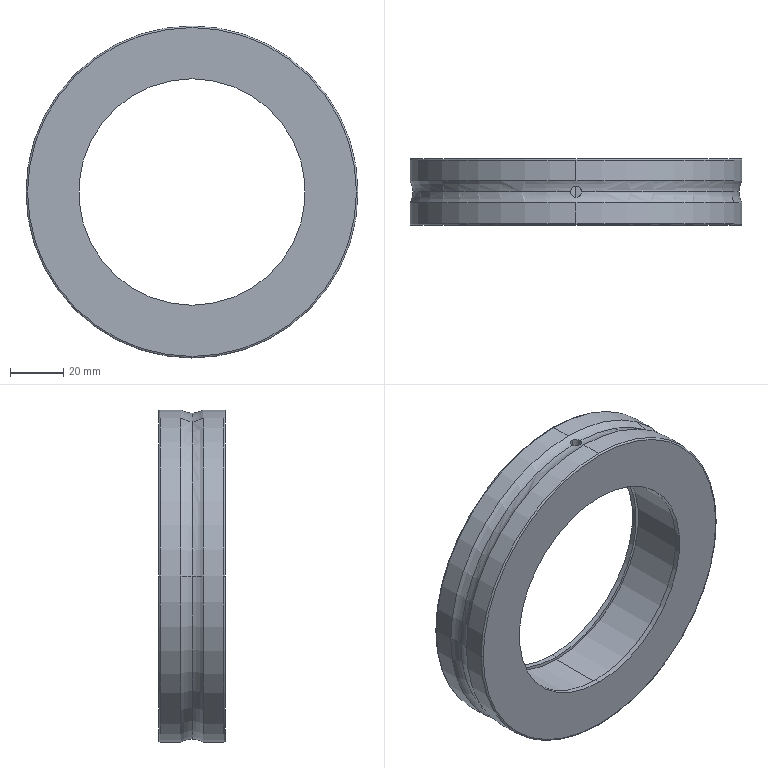Part | SolidWorks | features BaseBody 1 | 1 solid | 24 faces | box 125 x 25 x 125 mm | volume 154919 mm3 | cylinder 12 | torus 8 | plane 4 | commonest cylinder face diameters 85.25 x4 125 x4 4.159 x2 87.5 x2
STEP:
#1=CARTESIAN_POINT('',(-2132.95,755.069,-1534.999));
#2=VERTEX_POINT('',#1);
#3=CARTESIAN_POINT('',(-2132.95,755.069,-1620.249));
#4=VERTEX_POINT('',#3);
#5=CARTESIAN_POINT('',(-2132.95,755.069,-1577.624));
#6=DIRECTION('',(0.,-1.,0.));
#7=DIRECTION('',(0.,0.,1.));
#8=AXIS2_PLACEMENT_3D('',#5,#6,#7);
#9=CIRCLE('',#8,42.625);
#10=EDGE_CURVE('',#2,#4,#9,.T.);
#11=ORIENTED_EDGE('',*,*,#10,.F.);
#12=CARTESIAN_POINT('',(-2132.95,755.069,-1577.624));
#13=DIRECTION('',(0.,-1.,0.));
#14=DIRECTION('',(0.,0.,-1.));
#15=AXIS2_PLACEMENT_3D('',#12,#13,#14);
#16=CIRCLE('',#15,42.625);
#17=EDGE_CURVE('',#4,#2,#16,.T.);
#18=ORIENTED_EDGE('',*,*,#17,.F.);
#19=EDGE_LOOP('',(#11,#18));
#20=FACE_BOUND('',#19,.T.);
#21=CARTESIAN_POINT('',(-2071.05,755.069,-1577.624));
#22=VERTEX_POINT('',#21);
#23=CARTESIAN_POINT('',(-2194.85,755.069,-1577.624));
#24=VERTEX_POINT('',#23);
#25=CARTESIAN_POINT('',(-2132.95,755.069,-1577.624));
#26=DIRECTION('',(0.,-1.,0.));
#27=DIRECTION('',(0.,0.,1.));
#28=AXIS2_PLACEMENT_3D('',#25,#26,#27);
#29=CIRCLE('',#28,61.9);
#30=EDGE_CURVE('',#22,#24,#29,.T.);
#31=ORIENTED_EDGE('',*,*,#30,.T.);
#32=CARTESIAN_POINT('',(-2132.95,755.069,-1577.624));
#33=DIRECTION('',(0.,-1.,0.));
#34=DIRECTION('',(-1.,0.,0.));
#35=AXIS2_PLACEMENT_3D('',#32,#33,#34);
#36=CIRCLE('',#35,61.9);
#37=EDGE_CURVE('',#24,#22,#36,.T.);
#38=ORIENTED_EDGE('',*,*,#37,.T.);
#39=EDGE_LOOP('',(#31,#38));
#40=FACE_OUTER_BOUND('',#39,.T.);
#41=CARTESIAN_POINT('',(-2064.86,755.069,-1645.714));
#42=DIRECTION('',(0.,-1.,0.));
#43=DIRECTION('',(0.,0.,-1.));
#44=AXIS2_PLACEMENT_3D('',#41,#42,#43);
#45=PLANE('',#44);
#46=ADVANCED_FACE('',(#20,#40),#45,.T.);
#47=CARTESIAN_POINT('',(-2070.45,755.669,-1577.624));
#48=VERTEX_POINT('',#47);
#49=CARTESIAN_POINT('',(-2071.05,755.669,-1577.624));
#50=DIRECTION('',(0.,0.,-1.));
#51=DIRECTION('',(1.,0.,0.));
#52=AXIS2_PLACEMENT_3D('',#49,#50,#51);
#53=CIRCLE('',#52,0.6);
#54=EDGE_CURVE('',#48,#22,#53,.T.);
#55=ORIENTED_EDGE('',*,*,#54,.T.);
#56=ORIENTED_EDGE('',*,*,#37,.F.);
#57=CARTESIAN_POINT('',(-2195.45,755.669,-1577.624));
#58=VERTEX_POINT('',#57);
#59=CARTESIAN_POINT('',(-2194.85,755.669,-1577.624));
#60=DIRECTION('',(0.,0.,-1.));
#61=DIRECTION('',(0.,-1.,0.));
#62=AXIS2_PLACEMENT_3D('',#59,#60,#61);
#63=CIRCLE('',#62,0.6);
#64=EDGE_CURVE('',#24,#58,#63,.T.);
#65=ORIENTED_EDGE('',*,*,#64,.T.);
#66=CARTESIAN_POINT('',(-2132.95,755.669,-1640.124));
#67=VERTEX_POINT('',#66);
#68=CARTESIAN_POINT('',(-2132.95,755.669,-1577.624));
#69=DIRECTION('',(0.,-1.,0.));
#70=DIRECTION('',(-1.,0.,0.));
#71=AXIS2_PLACEMENT_3D('',#68,#69,#70);
#72=CIRCLE('',#71,62.5);
#73=EDGE_CURVE('',#58,#67,#72,.T.);
#74=ORIENTED_EDGE('',*,*,#73,.T.);
#75=CARTESIAN_POINT('',(-2132.95,755.669,-1577.624));
#76=DIRECTION('',(0.,-1.,0.));
#77=DIRECTION('',(0.,0.,-1.));
#78=AXIS2_PLACEMENT_3D('',#75,#76,#77);
#79=CIRCLE('',#78,62.5);
#80=EDGE_CURVE('',#67,#48,#79,.T.);
#81=ORIENTED_EDGE('',*,*,#80,.T.);
#82=EDGE_LOOP('',(#55,#56,#65,#74,#81));
#83=FACE_OUTER_BOUND('',#82,.T.);
#84=CARTESIAN_POINT('',(-2132.95,755.669,-1577.624));
#85=DIRECTION('',(0.,-1.,0.));
#86=DIRECTION('',(-0.9962,0.,0.08716));
#87=AXIS2_PLACEMENT_3D('',#84,#85,#86);
#88=TOROIDAL_SURFACE('',#87,61.9,0.6);
#89=ADVANCED_FACE('',(#83),#88,.T.);
#90=CARTESIAN_POINT('',(-2132.95,763.41,-1515.124));
#91=VERTEX_POINT('',#90);
#92=CARTESIAN_POINT('',(-2132.95,755.669,-1515.124));
#93=VERTEX_POINT('',#92);
#94=CARTESIAN_POINT('',(-2132.95,763.41,-1515.124));
#95=DIRECTION('',(0.,-1.,0.));
#96=VECTOR('',#95,1000.);
#97=LINE('',#94,#96);
#98=EDGE_CURVE('',#91,#93,#97,.T.);
#99=ORIENTED_EDGE('',*,*,#98,.T.);
#100=CARTESIAN_POINT('',(-2132.95,755.669,-1577.624));
#101=DIRECTION('',(0.,-1.,0.));
#102=DIRECTION('',(1.,0.,0.));
#103=AXIS2_PLACEMENT_3D('',#100,#101,#102);
#104=CIRCLE('',#103,62.5);
#105=EDGE_CURVE('',#48,#93,#104,.T.);
#106=ORIENTED_EDGE('',*,*,#105,.F.);
#107=ORIENTED_EDGE('',*,*,#80,.F.);
#108=CARTESIAN_POINT('',(-2132.95,763.41,-1640.124));
#109=VERTEX_POINT('',#108);
#110=CARTESIAN_POINT('',(-2132.95,755.669,-1640.124));
#111=DIRECTION('',(0.,1.,0.));
#112=VECTOR('',#111,1000.);
#113=LINE('',#110,#112);
#114=EDGE_CURVE('',#67,#109,#113,.T.);
#115=ORIENTED_EDGE('',*,*,#114,.T.);
#116=CARTESIAN_POINT('',(-2070.45,763.41,-1577.624));
#117=VERTEX_POINT('',#116);
#118=CARTESIAN_POINT('',(-2132.95,763.41,-1577.624));
#119=DIRECTION('',(0.,-1.,0.));
#120=DIRECTION('',(0.,0.,-1.));
#121=AXIS2_PLACEMENT_3D('',#118,#119,#120);
#122=CIRCLE('',#121,62.5);
#123=EDGE_CURVE('',#109,#117,#122,.T.);
#124=ORIENTED_EDGE('',*,*,#123,.T.);
#125=CARTESIAN_POINT('',(-2132.95,763.41,-1577.624));
#126=DIRECTION('',(0.,-1.,0.));
#127=DIRECTION('',(1.,0.,0.));
#128=AXIS2_PLACEMENT_3D('',#125,#126,#127);
#129=CIRCLE('',#128,62.5);
#130=EDGE_CURVE('',#117,#91,#129,.T.);
#131=ORIENTED_EDGE('',*,*,#130,.T.);
#132=EDGE_LOOP('',(#99,#106,#107,#115,#124,#131));
#133=FACE_OUTER_BOUND('',#132,.T.);
#134=CARTESIAN_POINT('',(-2132.95,763.797,-1577.624));
#135=DIRECTION('',(0.,1.,0.));
#136=DIRECTION('',(-0.08716,0.,0.9962));
#137=AXIS2_PLACEMENT_3D('',#134,#135,#136);
#138=CYLINDRICAL_SURFACE('',#137,62.5);
#139=ADVANCED_FACE('',(#133),#138,.T.);
#140=CARTESIAN_POINT('',(-2194.325,767.569,-1577.624));
#141=VERTEX_POINT('',#140);
#142=CARTESIAN_POINT('',(-2135.029,767.569,-1516.285));
#143=VERTEX_POINT('',#142);
#144=CARTESIAN_POINT('',(-2132.95,767.569,-1577.624));
#145=DIRECTION('',(0.,1.,0.));
#146=DIRECTION('',(-1.,0.,0.));
#147=AXIS2_PLACEMENT_3D('',#144,#145,#146);
#148=CIRCLE('',#147,61.375);
#149=EDGE_CURVE('',#141,#143,#148,.T.);
#150=ORIENTED_EDGE('',*,*,#149,.T.);
#151=CARTESIAN_POINT('',(-2132.95,769.648,-1515.983));
#152=VERTEX_POINT('',#151);
#153=CARTESIAN_POINT('',(-2135.029,767.569,-1516.285));
#154=CARTESIAN_POINT('',(-2135.029,767.706,-1516.285));
#155=CARTESIAN_POINT('',(-2135.016,767.842,-1516.281));
#156=CARTESIAN_POINT('',(-2134.963,768.108,-1516.266));
#157=CARTESIAN_POINT('',(-2134.923,768.239,-1516.255));
#158=CARTESIAN_POINT('',(-2134.765,768.62,-1516.213));
#159=CARTESIAN_POINT('',(-2134.616,768.843,-1516.175));
#160=CARTESIAN_POINT('',(-2134.323,769.136,-1516.115));
#161=CARTESIAN_POINT('',(-2134.218,769.222,-1516.095));
#162=CARTESIAN_POINT('',(-2133.994,769.372,-1516.059));
#163=CARTESIAN_POINT('',(-2133.876,769.436,-1516.042));
#164=CARTESIAN_POINT('',(-2133.491,769.595,-1515.999));
#165=CARTESIAN_POINT('',(-2133.225,769.648,-1515.983));
#166=CARTESIAN_POINT('',(-2132.95,769.648,-1515.983));
#167=B_SPLINE_CURVE_WITH_KNOTS('',3,(#153,#154,#155,#156,#157,#158,#159,#160,#161,#162,#163,#164,#165,#166),.UNSPECIFIED.,.F.,.F.,(4,2,2,2,2,2,4),(0.,0.125,0.25,0.5,0.625,0.75,1.),.UNSPECIFIED.);
#168=EDGE_CURVE('',#143,#152,#167,.T.);
#169=ORIENTED_EDGE('',*,*,#168,.T.);
#170=CARTESIAN_POINT('',(-2130.87,767.569,-1516.285));
#171=VERTEX_POINT('',#170);
#172=CARTESIAN_POINT('',(-2132.95,769.648,-1515.983));
#173=CARTESIAN_POINT('',(-2132.812,769.648,-1515.983));
#174=CARTESIAN_POINT('',(-2132.677,769.635,-1515.987));
#175=CARTESIAN_POINT('',(-2132.411,769.582,-1516.002));
#176=CARTESIAN_POINT('',(-2132.279,769.542,-1516.014));
#177=CARTESIAN_POINT('',(-2131.899,769.384,-1516.056));
#178=CARTESIAN_POINT('',(-2131.674,769.233,-1516.095));
#179=CARTESIAN_POINT('',(-2131.284,768.844,-1516.175));
#180=CARTESIAN_POINT('',(-2131.135,768.622,-1516.213));
#181=CARTESIAN_POINT('',(-2130.923,768.11,-1516.269));
#182=CARTESIAN_POINT('',(-2130.87,767.844,-1516.285));
#183=CARTESIAN_POINT('',(-2130.87,767.569,-1516.285));
#184=B_SPLINE_CURVE_WITH_KNOTS('',3,(#172,#173,#174,#175,#176,#177,#178,#179,#180,#181,#182,#183),.UNSPECIFIED.,.F.,.F.,(4,2,2,2,2,4),(0.,0.125,0.25,0.5,0.75,1.),.UNSPECIFIED.);
#185=EDGE_CURVE('',#152,#171,#184,.T.);
#186=ORIENTED_EDGE('',*,*,#185,.T.);
#187=CARTESIAN_POINT('',(-2071.575,767.569,-1577.624));
#188=VERTEX_POINT('',#187);
#189=CARTESIAN_POINT('',(-2132.95,767.569,-1577.624));
#190=DIRECTION('',(0.,1.,0.));
#191=DIRECTION('',(0.03388,0.,0.9994));
#192=AXIS2_PLACEMENT_3D('',#189,#190,#191);
#193=CIRCLE('',#192,61.375);
#194=EDGE_CURVE('',#171,#188,#193,.T.);
#195=ORIENTED_EDGE('',*,*,#194,.T.);
#196=CARTESIAN_POINT('',(-2070.45,771.727,-1577.624));
#197=VERTEX_POINT('',#196);
#198=CARTESIAN_POINT('',(-2063.325,767.569,-1577.624));
#199=DIRECTION('',(0.,0.,-1.));
#200=DIRECTION('',(-1.,0.,0.));
#201=AXIS2_PLACEMENT_3D('',#198,#199,#200);
#202=CIRCLE('',#201,8.25);
#203=EDGE_CURVE('',#188,#197,#202,.T.);
#204=ORIENTED_EDGE('',*,*,#203,.T.);
#205=CARTESIAN_POINT('',(-2132.95,771.727,-1515.124));
#206=VERTEX_POINT('',#205);
#207=CARTESIAN_POINT('',(-2132.95,771.727,-1577.624));
#208=DIRECTION('',(0.,-1.,0.));
#209=DIRECTION('',(1.,0.,0.));
#210=AXIS2_PLACEMENT_3D('',#207,#208,#209);
#211=CIRCLE('',#210,62.5);
#212=EDGE_CURVE('',#197,#206,#211,.T.);
#213=ORIENTED_EDGE('',*,*,#212,.T.);
#214=CARTESIAN_POINT('',(-2195.45,771.727,-1577.624));
#215=VERTEX_POINT('',#214);
#216=CARTESIAN_POINT('',(-2132.95,771.727,-1577.624));
#217=DIRECTION('',(0.,-1.,0.));
#218=DIRECTION('',(0.,0.,1.));
#219=AXIS2_PLACEMENT_3D('',#216,#217,#218);
#220=CIRCLE('',#219,62.5);
#221=EDGE_CURVE('',#206,#215,#220,.T.);
#222=ORIENTED_EDGE('',*,*,#221,.T.);
#223=CARTESIAN_POINT('',(-2202.575,767.569,-1577.624));
#224=DIRECTION('',(0.,0.,-1.));
#225=DIRECTION('',(0.8636,0.5041,0.));
#226=AXIS2_PLACEMENT_3D('',#223,#224,#225);
#227=CIRCLE('',#226,8.25);
#228=EDGE_CURVE('',#215,#141,#227,.T.);
#229=ORIENTED_EDGE('',*,*,#228,.T.);
#230=EDGE_LOOP('',(#150,#169,#186,#195,#204,#213,#222,#229));
#231=FACE_OUTER_BOUND('',#230,.T.);
#232=CARTESIAN_POINT('',(-2132.95,767.569,-1577.624));
#233=DIRECTION('',(0.,-1.,0.));
#234=DIRECTION('',(0.9962,0.,-0.08716));
#235=AXIS2_PLACEMENT_3D('',#232,#233,#234);
#236=TOROIDAL_SURFACE('',#235,69.625,8.25);
#237=ADVANCED_FACE('',(#231),#236,.F.);
#238=CARTESIAN_POINT('',(-2132.95,779.469,-1515.124));
#239=VERTEX_POINT('',#238);
#240=CARTESIAN_POINT('',(-2132.95,779.469,-1515.124));
#241=DIRECTION('',(0.,-1.,0.));
#242=VECTOR('',#241,1000.);
#243=LINE('',#240,#242);
#244=EDGE_CURVE('',#239,#206,#243,.T.);
#245=ORIENTED_EDGE('',*,*,#244,.T.);
#246=ORIENTED_EDGE('',*,*,#212,.F.);
#247=CARTESIAN_POINT('',(-2132.95,771.727,-1640.124));
#248=VERTEX_POINT('',#247);
#249=CARTESIAN_POINT('',(-2132.95,771.727,-1577.624));
#250=DIRECTION('',(0.,-1.,0.));
#251=DIRECTION('',(0.,0.,-1.));
#252=AXIS2_PLACEMENT_3D('',#249,#250,#251);
#253=CIRCLE('',#252,62.5);
#254=EDGE_CURVE('',#248,#197,#253,.T.);
#255=ORIENTED_EDGE('',*,*,#254,.F.);
#256=CARTESIAN_POINT('',(-2132.95,779.469,-1640.124));
#257=VERTEX_POINT('',#256);
#258=CARTESIAN_POINT('',(-2132.95,771.727,-1640.124));
#259=DIRECTION('',(0.,1.,0.));
#260=VECTOR('',#259,1000.);
#261=LINE('',#258,#260);
#262=EDGE_CURVE('',#248,#257,#261,.T.);
#263=ORIENTED_EDGE('',*,*,#262,.T.);
#264=CARTESIAN_POINT('',(-2070.45,779.469,-1577.624));
#265=VERTEX_POINT('',#264);
#266=CARTESIAN_POINT('',(-2132.95,779.469,-1577.624));
#267=DIRECTION('',(0.,-1.,0.));
#268=DIRECTION('',(0.,0.,-1.));
#269=AXIS2_PLACEMENT_3D('',#266,#267,#268);
#270=CIRCLE('',#269,62.5);
#271=EDGE_CURVE('',#257,#265,#270,.T.);
#272=ORIENTED_EDGE('',*,*,#271,.T.);
#273=CARTESIAN_POINT('',(-2132.95,779.469,-1577.624));
#274=DIRECTION('',(0.,-1.,0.));
#275=DIRECTION('',(1.,0.,0.));
#276=AXIS2_PLACEMENT_3D('',#273,#274,#275);
#277=CIRCLE('',#276,62.5);
#278=EDGE_CURVE('',#265,#239,#277,.T.);
#279=ORIENTED_EDGE('',*,*,#278,.T.);
#280=EDGE_LOOP('',(#245,#246,#255,#263,#272,#279));
#281=FACE_OUTER_BOUND('',#280,.T.);
#282=CARTESIAN_POINT('',(-2132.95,779.856,-1577.624));
#283=DIRECTION('',(0.,1.,0.));
#284=DIRECTION('',(-0.08716,0.,0.9962));
#285=AXIS2_PLACEMENT_3D('',#282,#283,#284);
#286=CYLINDRICAL_SURFACE('',#285,62.5);
#287=ADVANCED_FACE('',(#281),#286,.T.);
#288=CARTESIAN_POINT('',(-2071.05,780.069,-1577.624));
#289=VERTEX_POINT('',#288);
#290=CARTESIAN_POINT('',(-2071.05,779.469,-1577.624));
#291=DIRECTION('',(0.,0.,-1.));
#292=DIRECTION('',(0.,1.,0.));
#293=AXIS2_PLACEMENT_3D('',#290,#291,#292);
#294=CIRCLE('',#293,0.6);
#295=EDGE_CURVE('',#289,#265,#294,.T.);
#296=ORIENTED_EDGE('',*,*,#295,.T.);
#297=ORIENTED_EDGE('',*,*,#271,.F.);
#298=CARTESIAN_POINT('',(-2195.45,779.469,-1577.624));
#299=VERTEX_POINT('',#298);
#300=CARTESIAN_POINT('',(-2132.95,779.469,-1577.624));
#301=DIRECTION('',(0.,-1.,0.));
#302=DIRECTION('',(-1.,0.,0.));
#303=AXIS2_PLACEMENT_3D('',#300,#301,#302);
#304=CIRCLE('',#303,62.5);
#305=EDGE_CURVE('',#299,#257,#304,.T.);
#306=ORIENTED_EDGE('',*,*,#305,.F.);
#307=CARTESIAN_POINT('',(-2194.85,780.069,-1577.624));
#308=VERTEX_POINT('',#307);
#309=CARTESIAN_POINT('',(-2194.85,779.469,-1577.624));
#310=DIRECTION('',(0.,0.,-1.));
#311=DIRECTION('',(-1.,0.,0.));
#312=AXIS2_PLACEMENT_3D('',#309,#310,#311);
#313=CIRCLE('',#312,0.6);
#314=EDGE_CURVE('',#299,#308,#313,.T.);
#315=ORIENTED_EDGE('',*,*,#314,.T.);
#316=CARTESIAN_POINT('',(-2132.95,780.069,-1577.624));
#317=DIRECTION('',(0.,1.,0.));
#318=DIRECTION('',(1.,0.,0.));
#319=AXIS2_PLACEMENT_3D('',#316,#317,#318);
#320=CIRCLE('',#319,61.9);
#321=EDGE_CURVE('',#289,#308,#320,.T.);
#322=ORIENTED_EDGE('',*,*,#321,.F.);
#323=EDGE_LOOP('',(#296,#297,#306,#315,#322));
#324=FACE_OUTER_BOUND('',#323,.T.);
#325=CARTESIAN_POINT('',(-2132.95,779.469,-1577.624));
#326=DIRECTION('',(0.,-1.,0.));
#327=DIRECTION('',(-0.9962,0.,0.08716));
#328=AXIS2_PLACEMENT_3D('',#325,#326,#327);
#329=TOROIDAL_SURFACE('',#328,61.9,0.6);
#330=ADVANCED_FACE('',(#324),#329,.T.);
#331=CARTESIAN_POINT('',(-2132.95,780.069,-1620.249));
#332=VERTEX_POINT('',#331);
#333=CARTESIAN_POINT('',(-2132.95,780.069,-1534.999));
#334=VERTEX_POINT('',#333);
#335=CARTESIAN_POINT('',(-2132.95,780.069,-1577.624));
#336=DIRECTION('',(0.,1.,0.));
#337=DIRECTION('',(0.,0.,-1.));
#338=AXIS2_PLACEMENT_3D('',#335,#336,#337);
#339=CIRCLE('',#338,42.625);
#340=EDGE_CURVE('',#332,#334,#339,.T.);
#341=ORIENTED_EDGE('',*,*,#340,.F.);
#342=CARTESIAN_POINT('',(-2132.95,780.069,-1577.624));
#343=DIRECTION('',(0.,1.,0.));
#344=DIRECTION('',(0.,0.,1.));
#345=AXIS2_PLACEMENT_3D('',#342,#343,#344);
#346=CIRCLE('',#345,42.625);
#347=EDGE_CURVE('',#334,#332,#346,.T.);
#348=ORIENTED_EDGE('',*,*,#347,.F.);
#349=EDGE_LOOP('',(#341,#348));
#350=FACE_BOUND('',#349,.T.);
#351=CARTESIAN_POINT('',(-2132.95,780.069,-1577.624));
#352=DIRECTION('',(0.,1.,0.));
#353=DIRECTION('',(-1.,0.,0.));
#354=AXIS2_PLACEMENT_3D('',#351,#352,#353);
#355=CIRCLE('',#354,61.9);
#356=EDGE_CURVE('',#308,#289,#355,.T.);
#357=ORIENTED_EDGE('',*,*,#356,.T.);
#358=ORIENTED_EDGE('',*,*,#321,.T.);
#359=EDGE_LOOP('',(#357,#358));
#360=FACE_OUTER_BOUND('',#359,.T.);
#361=CARTESIAN_POINT('',(-2064.86,780.069,-1509.534));
#362=DIRECTION('',(0.,1.,0.));
#363=DIRECTION('',(1.,0.,0.));
#364=AXIS2_PLACEMENT_3D('',#361,#362,#363);
#365=PLANE('',#364);
#366=ADVANCED_FACE('',(#350,#360),#365,.T.);
#367=CARTESIAN_POINT('',(-2132.95,778.069,-1534.999));
#368=VERTEX_POINT('',#367);
#369=CARTESIAN_POINT('',(-2132.95,780.069,-1534.999));
#370=DIRECTION('',(0.,-1.,0.));
#371=VECTOR('',#370,1000.);
#372=LINE('',#369,#371);
#373=EDGE_CURVE('',#334,#368,#372,.T.);
#374=ORIENTED_EDGE('',*,*,#373,.T.);
#375=CARTESIAN_POINT('',(-2132.95,778.069,-1620.249));
#376=VERTEX_POINT('',#375);
#377=CARTESIAN_POINT('',(-2132.95,778.069,-1577.624));
#378=DIRECTION('',(0.,-1.,0.));
#379=DIRECTION('',(0.,0.,1.));
#380=AXIS2_PLACEMENT_3D('',#377,#378,#379);
#381=CIRCLE('',#380,42.625);
#382=EDGE_CURVE('',#368,#376,#381,.T.);
#383=ORIENTED_EDGE('',*,*,#382,.T.);
#384=CARTESIAN_POINT('',(-2132.95,778.069,-1620.249));
#385=DIRECTION('',(0.,1.,0.));
#386=VECTOR('',#385,1000.);
#387=LINE('',#384,#386);
#388=EDGE_CURVE('',#376,#332,#387,.T.);
#389=ORIENTED_EDGE('',*,*,#388,.T.);
#390=ORIENTED_EDGE('',*,*,#340,.T.);
#391=EDGE_LOOP('',(#374,#383,#389,#390));
#392=FACE_OUTER_BOUND('',#391,.T.);
#393=CARTESIAN_POINT('',(-2132.95,777.969,-1577.624));
#394=DIRECTION('',(0.,1.,0.));
#395=DIRECTION('',(0.08716,0.,-0.9962));
#396=AXIS2_PLACEMENT_3D('',#393,#394,#395);
#397=CYLINDRICAL_SURFACE('',#396,42.625);
#398=ADVANCED_FACE('',(#392),#397,.F.);
#399=ORIENTED_EDGE('',*,*,#382,.F.);
#400=CARTESIAN_POINT('',(-2132.95,778.069,-1577.624));
#401=DIRECTION('',(0.,-1.,0.));
#402=DIRECTION('',(0.,0.,-1.));
#403=AXIS2_PLACEMENT_3D('',#400,#401,#402);
#404=CIRCLE('',#403,42.625);
#405=EDGE_CURVE('',#376,#368,#404,.T.);
#406=ORIENTED_EDGE('',*,*,#405,.F.);
#407=EDGE_LOOP('',(#399,#406));
#408=FACE_BOUND('',#407,.T.);
#409=CARTESIAN_POINT('',(-2132.95,778.069,-1533.874));
#410=VERTEX_POINT('',#409);
#411=CARTESIAN_POINT('',(-2132.95,778.069,-1621.374));
#412=VERTEX_POINT('',#411);
#413=CARTESIAN_POINT('',(-2132.95,778.069,-1577.624));
#414=DIRECTION('',(0.,-1.,0.));
#415=DIRECTION('',(0.,0.,1.));
#416=AXIS2_PLACEMENT_3D('',#413,#414,#415);
#417=CIRCLE('',#416,43.75);
#418=EDGE_CURVE('',#410,#412,#417,.T.);
#419=ORIENTED_EDGE('',*,*,#418,.T.);
#420=CARTESIAN_POINT('',(-2132.95,778.069,-1577.624));
#421=DIRECTION('',(0.,-1.,0.));
#422=DIRECTION('',(0.,0.,-1.));
#423=AXIS2_PLACEMENT_3D('',#420,#421,#422);
#424=CIRCLE('',#423,43.75);
#425=EDGE_CURVE('',#412,#410,#424,.T.);
#426=ORIENTED_EDGE('',*,*,#425,.T.);
#427=EDGE_LOOP('',(#419,#426));
#428=FACE_OUTER_BOUND('',#427,.T.);
#429=CARTESIAN_POINT('',(-2084.864,778.069,-1625.749));
#430=DIRECTION('',(0.,-1.,0.));
#431=DIRECTION('',(0.,0.,-1.));
#432=AXIS2_PLACEMENT_3D('',#429,#430,#431);
#433=PLANE('',#432);
#434=ADVANCED_FACE('',(#408,#428),#433,.T.);
#435=CARTESIAN_POINT('',(-2132.95,769.648,-1533.874));
#436=VERTEX_POINT('',#435);
#437=CARTESIAN_POINT('',(-2132.95,778.069,-1533.874));
#438=DIRECTION('',(0.,-1.,0.));
#439=VECTOR('',#438,1000.);
#440=LINE('',#437,#439);
#441=EDGE_CURVE('',#410,#436,#440,.T.);
#442=ORIENTED_EDGE('',*,*,#441,.T.);
#443=CARTESIAN_POINT('',(-2132.95,765.489,-1533.874));
#444=VERTEX_POINT('',#443);
#445=CARTESIAN_POINT('',(-2132.95,769.648,-1533.874));
#446=CARTESIAN_POINT('',(-2133.225,769.648,-1533.874));
#447=CARTESIAN_POINT('',(-2133.489,769.596,-1533.877));
#448=CARTESIAN_POINT('',(-2133.999,769.385,-1533.886));
#449=CARTESIAN_POINT('',(-2134.225,769.234,-1533.893));
#450=CARTESIAN_POINT('',(-2134.615,768.844,-1533.906));
#451=CARTESIAN_POINT('',(-2134.765,768.619,-1533.912));
#452=CARTESIAN_POINT('',(-2134.976,768.11,-1533.921));
#453=CARTESIAN_POINT('',(-2135.029,767.844,-1533.924));
#454=CARTESIAN_POINT('',(-2135.029,767.293,-1533.924));
#455=CARTESIAN_POINT('',(-2134.976,767.027,-1533.921));
#456=CARTESIAN_POINT('',(-2134.765,766.518,-1533.912));
#457=CARTESIAN_POINT('',(-2134.615,766.293,-1533.906));
#458=CARTESIAN_POINT('',(-2134.225,765.903,-1533.893));
#459=CARTESIAN_POINT('',(-2133.999,765.752,-1533.886));
#460=CARTESIAN_POINT('',(-2133.49,765.542,-1533.877));
#461=CARTESIAN_POINT('',(-2133.225,765.489,-1533.874));
#462=CARTESIAN_POINT('',(-2132.95,765.489,-1533.874));
#463=B_SPLINE_CURVE_WITH_KNOTS('',3,(#445,#446,#447,#448,#449,#450,#451,#452,#453,#454,#455,#456,#457,#458,#459,#460,#461,#462),.UNSPECIFIED.,.F.,.F.,(4,2,2,2,2,2,2,2,4),(0.,0.125,0.25,0.375,0.5,0.625,0.75,0.875,1.),.UNSPECIFIED.);
#464=EDGE_CURVE('',#436,#444,#463,.T.);
#465=ORIENTED_EDGE('',*,*,#464,.T.);
#466=CARTESIAN_POINT('',(-2132.95,757.069,-1533.874));
#467=VERTEX_POINT('',#466);
#468=CARTESIAN_POINT('',(-2132.95,765.489,-1533.874));
#469=DIRECTION('',(0.,-1.,0.));
#470=VECTOR('',#469,1000.);
#471=LINE('',#468,#470);
#472=EDGE_CURVE('',#444,#467,#471,.T.);
#473=ORIENTED_EDGE('',*,*,#472,.T.);
#474=CARTESIAN_POINT('',(-2132.95,757.069,-1621.374));
#475=VERTEX_POINT('',#474);
#476=CARTESIAN_POINT('',(-2132.95,757.069,-1577.624));
#477=DIRECTION('',(0.,1.,0.));
#478=DIRECTION('',(0.,0.,-1.));
#479=AXIS2_PLACEMENT_3D('',#476,#477,#478);
#480=CIRCLE('',#479,43.75);
#481=EDGE_CURVE('',#475,#467,#480,.T.);
#482=ORIENTED_EDGE('',*,*,#481,.F.);
#483=CARTESIAN_POINT('',(-2132.95,757.069,-1621.374));
#484=DIRECTION('',(0.,1.,0.));
#485=VECTOR('',#484,1000.);
#486=LINE('',#483,#485);
#487=EDGE_CURVE('',#475,#412,#486,.T.);
#488=ORIENTED_EDGE('',*,*,#487,.T.);
#489=ORIENTED_EDGE('',*,*,#418,.F.);
#490=EDGE_LOOP('',(#442,#465,#473,#482,#488,#489));
#491=FACE_OUTER_BOUND('',#490,.T.);
#492=CARTESIAN_POINT('',(-2132.95,756.019,-1577.624));
#493=DIRECTION('',(0.,1.,0.));
#494=DIRECTION('',(0.08716,0.,-0.9962));
#495=AXIS2_PLACEMENT_3D('',#492,#493,#494);
#496=CYLINDRICAL_SURFACE('',#495,43.75);
#497=ADVANCED_FACE('',(#491),#496,.F.);
#498=CARTESIAN_POINT('',(-2132.95,757.069,-1620.249));
#499=VERTEX_POINT('',#498);
#500=CARTESIAN_POINT('',(-2132.95,757.069,-1534.999));
#501=VERTEX_POINT('',#500);
#502=CARTESIAN_POINT('',(-2132.95,757.069,-1577.624));
#503=DIRECTION('',(0.,1.,0.));
#504=DIRECTION('',(0.,0.,-1.));
#505=AXIS2_PLACEMENT_3D('',#502,#503,#504);
#506=CIRCLE('',#505,42.625);
#507=EDGE_CURVE('',#499,#501,#506,.T.);
#508=ORIENTED_EDGE('',*,*,#507,.F.);
#509=CARTESIAN_POINT('',(-2132.95,757.069,-1577.624));
#510=DIRECTION('',(0.,1.,0.));
#511=DIRECTION('',(0.,0.,1.));
#512=AXIS2_PLACEMENT_3D('',#509,#510,#511);
#513=CIRCLE('',#512,42.625);
#514=EDGE_CURVE('',#501,#499,#513,.T.);
#515=ORIENTED_EDGE('',*,*,#514,.F.);
#516=EDGE_LOOP('',(#508,#515));
#517=FACE_BOUND('',#516,.T.);
#518=ORIENTED_EDGE('',*,*,#481,.T.);
#519=CARTESIAN_POINT('',(-2132.95,757.069,-1577.624));
#520=DIRECTION('',(0.,1.,0.));
#521=DIRECTION('',(0.,0.,1.));
#522=AXIS2_PLACEMENT_3D('',#519,#520,#521);
#523=CIRCLE('',#522,43.75);
#524=EDGE_CURVE('',#467,#475,#523,.T.);
#525=ORIENTED_EDGE('',*,*,#524,.T.);
#526=EDGE_LOOP('',(#518,#525));
#527=FACE_OUTER_BOUND('',#526,.T.);
#528=CARTESIAN_POINT('',(-2084.864,757.069,-1529.499));
#529=DIRECTION('',(0.,1.,0.));
#530=DIRECTION('',(1.,0.,0.));
#531=AXIS2_PLACEMENT_3D('',#528,#529,#530);
#532=PLANE('',#531);
#533=ADVANCED_FACE('',(#517,#527),#532,.T.);
#534=CARTESIAN_POINT('',(-2132.95,757.069,-1534.999));
#535=DIRECTION('',(0.,-1.,0.));
#536=VECTOR('',#535,1000.);
#537=LINE('',#534,#536);
#538=EDGE_CURVE('',#501,#2,#537,.T.);
#539=ORIENTED_EDGE('',*,*,#538,.T.);
#540=ORIENTED_EDGE('',*,*,#10,.T.);
#541=CARTESIAN_POINT('',(-2132.95,755.069,-1620.249));
#542=DIRECTION('',(0.,1.,0.));
#543=VECTOR('',#542,1000.);
#544=LINE('',#541,#543);
#545=EDGE_CURVE('',#4,#499,#544,.T.);
#546=ORIENTED_EDGE('',*,*,#545,.T.);
#547=ORIENTED_EDGE('',*,*,#507,.T.);
#548=EDGE_LOOP('',(#539,#540,#546,#547));
#549=FACE_OUTER_BOUND('',#548,.T.);
#550=CARTESIAN_POINT('',(-2132.95,754.969,-1577.624));
#551=DIRECTION('',(0.,1.,0.));
#552=DIRECTION('',(0.08716,0.,-0.9962));
#553=AXIS2_PLACEMENT_3D('',#550,#551,#552);
#554=CYLINDRICAL_SURFACE('',#553,42.625);
#555=ADVANCED_FACE('',(#549),#554,.F.);
#556=CARTESIAN_POINT('',(-2132.95,769.648,-1533.874));
#557=DIRECTION('',(0.,0.,1.));
#558=VECTOR('',#557,1000.);
#559=LINE('',#556,#558);
#560=EDGE_CURVE('',#436,#152,#559,.T.);
#561=ORIENTED_EDGE('',*,*,#560,.T.);
#562=ORIENTED_EDGE('',*,*,#168,.F.);
#563=CARTESIAN_POINT('',(-2132.95,765.489,-1515.983));
#564=VERTEX_POINT('',#563);
#565=CARTESIAN_POINT('',(-2132.95,765.489,-1515.983));
#566=CARTESIAN_POINT('',(-2133.087,765.489,-1515.983));
#567=CARTESIAN_POINT('',(-2133.223,765.502,-1515.987));
#568=CARTESIAN_POINT('',(-2133.489,765.555,-1516.002));
#569=CARTESIAN_POINT('',(-2133.621,765.595,-1516.014));
#570=CARTESIAN_POINT('',(-2134.001,765.753,-1516.056));
#571=CARTESIAN_POINT('',(-2134.226,765.904,-1516.095));
#572=CARTESIAN_POINT('',(-2134.518,766.196,-1516.155));
#573=CARTESIAN_POINT('',(-2134.604,766.3,-1516.174));
#574=CARTESIAN_POINT('',(-2134.754,766.525,-1516.21));
#575=CARTESIAN_POINT('',(-2134.817,766.643,-1516.227));
#576=CARTESIAN_POINT('',(-2134.976,767.027,-1516.269));
#577=CARTESIAN_POINT('',(-2135.029,767.293,-1516.285));
#578=CARTESIAN_POINT('',(-2135.029,767.569,-1516.285));
#579=B_SPLINE_CURVE_WITH_KNOTS('',3,(#565,#566,#567,#568,#569,#570,#571,#572,#573,#574,#575,#576,#577,#578),.UNSPECIFIED.,.F.,.F.,(4,2,2,2,2,2,4),(0.,0.125,0.25,0.5,0.625,0.75,1.),.UNSPECIFIED.);
#580=EDGE_CURVE('',#564,#143,#579,.T.);
#581=ORIENTED_EDGE('',*,*,#580,.F.);
#582=CARTESIAN_POINT('',(-2132.95,765.489,-1515.983));
#583=DIRECTION('',(0.,0.,-1.));
#584=VECTOR('',#583,1000.);
#585=LINE('',#582,#584);
#586=EDGE_CURVE('',#564,#444,#585,.T.);
#587=ORIENTED_EDGE('',*,*,#586,.T.);
#588=ORIENTED_EDGE('',*,*,#464,.F.);
#589=EDGE_LOOP('',(#561,#562,#581,#587,#588));
#590=FACE_OUTER_BOUND('',#589,.T.);
#591=CARTESIAN_POINT('',(-2132.95,767.569,-1534.821));
#592=DIRECTION('',(0.,0.,1.));
#593=DIRECTION('',(0.08716,0.9962,0.));
#594=AXIS2_PLACEMENT_3D('',#591,#592,#593);
#595=CYLINDRICAL_SURFACE('',#594,2.079);
#596=ADVANCED_FACE('',(#590),#595,.F.);
#597=ORIENTED_EDGE('',*,*,#560,.F.);
#598=CARTESIAN_POINT('',(-2130.87,767.569,-1533.924));
#599=VERTEX_POINT('',#598);
#600=CARTESIAN_POINT('',(-2130.87,767.569,-1533.924));
#601=CARTESIAN_POINT('',(-2130.87,767.844,-1533.924));
#602=CARTESIAN_POINT('',(-2130.923,768.109,-1533.921));
#603=CARTESIAN_POINT('',(-2131.134,768.619,-1533.912));
#604=CARTESIAN_POINT('',(-2131.284,768.844,-1533.906));
#605=CARTESIAN_POINT('',(-2131.674,769.234,-1533.893));
#606=CARTESIAN_POINT('',(-2131.9,769.384,-1533.886));
#607=CARTESIAN_POINT('',(-2132.409,769.595,-1533.877));
#608=CARTESIAN_POINT('',(-2132.674,769.648,-1533.874));
#609=CARTESIAN_POINT('',(-2132.95,769.648,-1533.874));
#610=B_SPLINE_CURVE_WITH_KNOTS('',3,(#600,#601,#602,#603,#604,#605,#606,#607,#608,#609),.UNSPECIFIED.,.F.,.F.,(4,2,2,2,4),(0.,0.25,0.5,0.75,1.),.UNSPECIFIED.);
#611=EDGE_CURVE('',#599,#436,#610,.T.);
#612=ORIENTED_EDGE('',*,*,#611,.F.);
#613=CARTESIAN_POINT('',(-2132.95,765.489,-1533.874));
#614=CARTESIAN_POINT('',(-2132.674,765.489,-1533.874));
#615=CARTESIAN_POINT('',(-2132.41,765.542,-1533.877));
#616=CARTESIAN_POINT('',(-2131.899,765.753,-1533.886));
#617=CARTESIAN_POINT('',(-2131.674,765.903,-1533.893));
#618=CARTESIAN_POINT('',(-2131.284,766.293,-1533.906));
#619=CARTESIAN_POINT('',(-2131.134,766.519,-1533.912));
#620=CARTESIAN_POINT('',(-2130.923,767.028,-1533.921));
#621=CARTESIAN_POINT('',(-2130.87,767.293,-1533.924));
#622=CARTESIAN_POINT('',(-2130.87,767.569,-1533.924));
#623=B_SPLINE_CURVE_WITH_KNOTS('',3,(#613,#614,#615,#616,#617,#618,#619,#620,#621,#622),.UNSPECIFIED.,.F.,.F.,(4,2,2,2,4),(0.,0.25,0.5,0.75,1.),.UNSPECIFIED.);
#624=EDGE_CURVE('',#444,#599,#623,.T.);
#625=ORIENTED_EDGE('',*,*,#624,.F.);
#626=ORIENTED_EDGE('',*,*,#586,.F.);
#627=CARTESIAN_POINT('',(-2130.87,767.569,-1516.285));
#628=CARTESIAN_POINT('',(-2130.87,767.431,-1516.285));
#629=CARTESIAN_POINT('',(-2130.883,767.295,-1516.281));
#630=CARTESIAN_POINT('',(-2130.936,767.029,-1516.266));
#631=CARTESIAN_POINT('',(-2130.977,766.898,-1516.255));
#632=CARTESIAN_POINT('',(-2131.135,766.517,-1516.213));
#633=CARTESIAN_POINT('',(-2131.284,766.294,-1516.175));
#634=CARTESIAN_POINT('',(-2131.577,766.001,-1516.115));
#635=CARTESIAN_POINT('',(-2131.681,765.915,-1516.095));
#636=CARTESIAN_POINT('',(-2131.906,765.765,-1516.059));
#637=CARTESIAN_POINT('',(-2132.024,765.701,-1516.042));
#638=CARTESIAN_POINT('',(-2132.408,765.542,-1515.999));
#639=CARTESIAN_POINT('',(-2132.674,765.489,-1515.983));
#640=CARTESIAN_POINT('',(-2132.95,765.489,-1515.983));
#641=B_SPLINE_CURVE_WITH_KNOTS('',3,(#627,#628,#629,#630,#631,#632,#633,#634,#635,#636,#637,#638,#639,#640),.UNSPECIFIED.,.F.,.F.,(4,2,2,2,2,2,4),(0.,0.125,0.25,0.5,0.625,0.75,1.),.UNSPECIFIED.);
#642=EDGE_CURVE('',#171,#564,#641,.T.);
#643=ORIENTED_EDGE('',*,*,#642,.F.);
#644=ORIENTED_EDGE('',*,*,#185,.F.);
#645=EDGE_LOOP('',(#597,#612,#625,#626,#643,#644));
#646=FACE_OUTER_BOUND('',#645,.T.);
#647=CARTESIAN_POINT('',(-2132.95,767.569,-1534.821));
#648=DIRECTION('',(0.,0.,1.));
#649=DIRECTION('',(-0.08716,-0.9962,0.));
#650=AXIS2_PLACEMENT_3D('',#647,#648,#649);
#651=CYLINDRICAL_SURFACE('',#650,2.079);
#652=ADVANCED_FACE('',(#646),#651,.F.);
#653=ORIENTED_EDGE('',*,*,#538,.F.);
#654=ORIENTED_EDGE('',*,*,#514,.T.);
#655=ORIENTED_EDGE('',*,*,#545,.F.);
#656=ORIENTED_EDGE('',*,*,#17,.T.);
#657=EDGE_LOOP('',(#653,#654,#655,#656));
#658=FACE_OUTER_BOUND('',#657,.T.);
#659=CARTESIAN_POINT('',(-2132.95,754.969,-1577.624));
#660=DIRECTION('',(0.,1.,0.));
#661=DIRECTION('',(-0.08716,0.,0.9962));
#662=AXIS2_PLACEMENT_3D('',#659,#660,#661);
#663=CYLINDRICAL_SURFACE('',#662,42.625);
#664=ADVANCED_FACE('',(#658),#663,.F.);
#665=ORIENTED_EDGE('',*,*,#441,.F.);
#666=ORIENTED_EDGE('',*,*,#425,.F.);
#667=ORIENTED_EDGE('',*,*,#487,.F.);
#668=ORIENTED_EDGE('',*,*,#524,.F.);
#669=ORIENTED_EDGE('',*,*,#472,.F.);
#670=ORIENTED_EDGE('',*,*,#624,.T.);
#671=ORIENTED_EDGE('',*,*,#611,.T.);
#672=EDGE_LOOP('',(#665,#666,#667,#668,#669,#670,#671));
#673=FACE_OUTER_BOUND('',#672,.T.);
#674=CARTESIAN_POINT('',(-2132.95,756.019,-1577.624));
#675=DIRECTION('',(0.,1.,0.));
#676=DIRECTION('',(-0.08716,0.,0.9962));
#677=AXIS2_PLACEMENT_3D('',#674,#675,#676);
#678=CYLINDRICAL_SURFACE('',#677,43.75);
#679=ADVANCED_FACE('',(#673),#678,.F.);
#680=ORIENTED_EDGE('',*,*,#373,.F.);
#681=ORIENTED_EDGE('',*,*,#347,.T.);
#682=ORIENTED_EDGE('',*,*,#388,.F.);
#683=ORIENTED_EDGE('',*,*,#405,.T.);
#684=EDGE_LOOP('',(#680,#681,#682,#683));
#685=FACE_OUTER_BOUND('',#684,.T.);
#686=CARTESIAN_POINT('',(-2132.95,777.969,-1577.624));
#687=DIRECTION('',(0.,1.,0.));
#688=DIRECTION('',(-0.08716,0.,0.9962));
#689=AXIS2_PLACEMENT_3D('',#686,#687,#688);
#690=CYLINDRICAL_SURFACE('',#689,42.625);
#691=ADVANCED_FACE('',(#685),#690,.F.);
#692=ORIENTED_EDGE('',*,*,#295,.F.);
#693=ORIENTED_EDGE('',*,*,#356,.F.);
#694=ORIENTED_EDGE('',*,*,#314,.F.);
#695=CARTESIAN_POINT('',(-2132.95,779.469,-1577.624));
#696=DIRECTION('',(0.,-1.,0.));
#697=DIRECTION('',(0.,0.,1.));
#698=AXIS2_PLACEMENT_3D('',#695,#696,#697);
#699=CIRCLE('',#698,62.5);
#700=EDGE_CURVE('',#239,#299,#699,.T.);
#701=ORIENTED_EDGE('',*,*,#700,.F.);
#702=ORIENTED_EDGE('',*,*,#278,.F.);
#703=EDGE_LOOP('',(#692,#693,#694,#701,#702));
#704=FACE_OUTER_BOUND('',#703,.T.);
#705=CARTESIAN_POINT('',(-2132.95,779.469,-1577.624));
#706=DIRECTION('',(0.,-1.,0.));
#707=DIRECTION('',(0.9962,0.,-0.08716));
#708=AXIS2_PLACEMENT_3D('',#705,#706,#707);
#709=TOROIDAL_SURFACE('',#708,61.9,0.6);
#710=ADVANCED_FACE('',(#704),#709,.T.);
#711=ORIENTED_EDGE('',*,*,#244,.F.);
#712=ORIENTED_EDGE('',*,*,#700,.T.);
#713=ORIENTED_EDGE('',*,*,#305,.T.);
#714=ORIENTED_EDGE('',*,*,#262,.F.);
#715=CARTESIAN_POINT('',(-2132.95,771.727,-1577.624));
#716=DIRECTION('',(0.,-1.,0.));
#717=DIRECTION('',(-1.,0.,0.));
#718=AXIS2_PLACEMENT_3D('',#715,#716,#717);
#719=CIRCLE('',#718,62.5);
#720=EDGE_CURVE('',#215,#248,#719,.T.);
#721=ORIENTED_EDGE('',*,*,#720,.F.);
#722=ORIENTED_EDGE('',*,*,#221,.F.);
#723=EDGE_LOOP('',(#711,#712,#713,#714,#721,#722));
#724=FACE_OUTER_BOUND('',#723,.T.);
#725=CARTESIAN_POINT('',(-2132.95,779.856,-1577.624));
#726=DIRECTION('',(0.,1.,0.));
#727=DIRECTION('',(0.08716,0.,-0.9962));
#728=AXIS2_PLACEMENT_3D('',#725,#726,#727);
#729=CYLINDRICAL_SURFACE('',#728,62.5);
#730=ADVANCED_FACE('',(#724),#729,.T.);
#731=CARTESIAN_POINT('',(-2132.95,767.569,-1577.624));
#732=DIRECTION('',(0.,1.,0.));
#733=DIRECTION('',(1.,0.,0.));
#734=AXIS2_PLACEMENT_3D('',#731,#732,#733);
#735=CIRCLE('',#734,61.375);
#736=EDGE_CURVE('',#188,#141,#735,.T.);
#737=ORIENTED_EDGE('',*,*,#736,.T.);
#738=ORIENTED_EDGE('',*,*,#228,.F.);
#739=ORIENTED_EDGE('',*,*,#720,.T.);
#740=ORIENTED_EDGE('',*,*,#254,.T.);
#741=ORIENTED_EDGE('',*,*,#203,.F.);
#742=EDGE_LOOP('',(#737,#738,#739,#740,#741));
#743=FACE_OUTER_BOUND('',#742,.T.);
#744=CARTESIAN_POINT('',(-2132.95,767.569,-1577.624));
#745=DIRECTION('',(0.,-1.,0.));
#746=DIRECTION('',(-0.9962,0.,0.08716));
#747=AXIS2_PLACEMENT_3D('',#744,#745,#746);
#748=TOROIDAL_SURFACE('',#747,69.625,8.25);
#749=ADVANCED_FACE('',(#743),#748,.F.);
#750=ORIENTED_EDGE('',*,*,#98,.F.);
#751=CARTESIAN_POINT('',(-2195.45,763.41,-1577.624));
#752=VERTEX_POINT('',#751);
#753=CARTESIAN_POINT('',(-2132.95,763.41,-1577.624));
#754=DIRECTION('',(0.,-1.,0.));
#755=DIRECTION('',(0.,0.,1.));
#756=AXIS2_PLACEMENT_3D('',#753,#754,#755);
#757=CIRCLE('',#756,62.5);
#758=EDGE_CURVE('',#91,#752,#757,.T.);
#759=ORIENTED_EDGE('',*,*,#758,.T.);
#760=CARTESIAN_POINT('',(-2132.95,763.41,-1577.624));
#761=DIRECTION('',(0.,-1.,0.));
#762=DIRECTION('',(-1.,0.,0.));
#763=AXIS2_PLACEMENT_3D('',#760,#761,#762);
#764=CIRCLE('',#763,62.5);
#765=EDGE_CURVE('',#752,#109,#764,.T.);
#766=ORIENTED_EDGE('',*,*,#765,.T.);
#767=ORIENTED_EDGE('',*,*,#114,.F.);
#768=ORIENTED_EDGE('',*,*,#73,.F.);
#769=CARTESIAN_POINT('',(-2132.95,755.669,-1577.624));
#770=DIRECTION('',(0.,-1.,0.));
#771=DIRECTION('',(0.,0.,1.));
#772=AXIS2_PLACEMENT_3D('',#769,#770,#771);
#773=CIRCLE('',#772,62.5);
#774=EDGE_CURVE('',#93,#58,#773,.T.);
#775=ORIENTED_EDGE('',*,*,#774,.F.);
#776=EDGE_LOOP('',(#750,#759,#766,#767,#768,#775));
#777=FACE_OUTER_BOUND('',#776,.T.);
#778=CARTESIAN_POINT('',(-2132.95,763.797,-1577.624));
#779=DIRECTION('',(0.,1.,0.));
#780=DIRECTION('',(0.08716,0.,-0.9962));
#781=AXIS2_PLACEMENT_3D('',#778,#779,#780);
#782=CYLINDRICAL_SURFACE('',#781,62.5);
#783=ADVANCED_FACE('',(#777),#782,.T.);
#784=ORIENTED_EDGE('',*,*,#54,.F.);
#785=ORIENTED_EDGE('',*,*,#105,.T.);
#786=ORIENTED_EDGE('',*,*,#774,.T.);
#787=ORIENTED_EDGE('',*,*,#64,.F.);
#788=ORIENTED_EDGE('',*,*,#30,.F.);
#789=EDGE_LOOP('',(#784,#785,#786,#787,#788));
#790=FACE_OUTER_BOUND('',#789,.T.);
#791=CARTESIAN_POINT('',(-2132.95,755.669,-1577.624));
#792=DIRECTION('',(0.,-1.,0.));
#793=DIRECTION('',(0.9962,0.,-0.08716));
#794=AXIS2_PLACEMENT_3D('',#791,#792,#793);
#795=TOROIDAL_SURFACE('',#794,61.9,0.6);
#796=ADVANCED_FACE('',(#790),#795,.T.);
#797=ORIENTED_EDGE('',*,*,#736,.F.);
#798=CARTESIAN_POINT('',(-2063.325,767.569,-1577.624));
#799=DIRECTION('',(0.,0.,-1.));
#800=DIRECTION('',(-0.8636,-0.5041,0.));
#801=AXIS2_PLACEMENT_3D('',#798,#799,#800);
#802=CIRCLE('',#801,8.25);
#803=EDGE_CURVE('',#117,#188,#802,.T.);
#804=ORIENTED_EDGE('',*,*,#803,.F.);
#805=ORIENTED_EDGE('',*,*,#123,.F.);
#806=ORIENTED_EDGE('',*,*,#765,.F.);
#807=CARTESIAN_POINT('',(-2202.575,767.569,-1577.624));
#808=DIRECTION('',(0.,0.,-1.));
#809=DIRECTION('',(1.,0.,0.));
#810=AXIS2_PLACEMENT_3D('',#807,#808,#809);
#811=CIRCLE('',#810,8.25);
#812=EDGE_CURVE('',#141,#752,#811,.T.);
#813=ORIENTED_EDGE('',*,*,#812,.F.);
#814=EDGE_LOOP('',(#797,#804,#805,#806,#813));
#815=FACE_OUTER_BOUND('',#814,.T.);
#816=CARTESIAN_POINT('',(-2132.95,767.569,-1577.624));
#817=DIRECTION('',(0.,-1.,0.));
#818=DIRECTION('',(-0.9962,0.,0.08716));
#819=AXIS2_PLACEMENT_3D('',#816,#817,#818);
#820=TOROIDAL_SURFACE('',#819,69.625,8.25);
#821=ADVANCED_FACE('',(#815),#820,.F.);
#822=ORIENTED_EDGE('',*,*,#149,.F.);
#823=ORIENTED_EDGE('',*,*,#812,.T.);
#824=ORIENTED_EDGE('',*,*,#758,.F.);
#825=ORIENTED_EDGE('',*,*,#130,.F.);
#826=ORIENTED_EDGE('',*,*,#803,.T.);
#827=ORIENTED_EDGE('',*,*,#194,.F.);
#828=ORIENTED_EDGE('',*,*,#642,.T.);
#829=ORIENTED_EDGE('',*,*,#580,.T.);
#830=EDGE_LOOP('',(#822,#823,#824,#825,#826,#827,#828,#829));
#831=FACE_OUTER_BOUND('',#830,.T.);
#832=CARTESIAN_POINT('',(-2132.95,767.569,-1577.624));
#833=DIRECTION('',(0.,-1.,0.));
#834=DIRECTION('',(0.9962,0.,-0.08716));
#835=AXIS2_PLACEMENT_3D('',#832,#833,#834);
#836=TOROIDAL_SURFACE('',#835,69.625,8.25);
#837=ADVANCED_FACE('',(#831),#836,.F.);
#838=CLOSED_SHELL('',(#46,#89,#139,#237,#287,#330,#366,#398,#434,#497,#533,#555,#596,#652,#664,#679,#691,#710,#730,#749,#783,#796,#821,#837));
#839=MANIFOLD_SOLID_BREP('',#838);
#840=CARTESIAN_POINT('',(0.,0.,0.));
#841=DIRECTION('',(0.,0.,1.));
#842=DIRECTION('',(1.,0.,0.));
#843=AXIS2_PLACEMENT_3D('',#840,#841,#842);
#844=(LENGTH_UNIT()NAMED_UNIT(*)SI_UNIT(.MILLI.,.METRE.));
#845=UNCERTAINTY_MEASURE_WITH_UNIT(LENGTH_MEASURE(0.00001),#844,'','');
#846=(NAMED_UNIT(*)PLANE_ANGLE_UNIT()SI_UNIT($,.RADIAN.));
#847=(NAMED_UNIT(*)SI_UNIT($,.STERADIAN.)SOLID_ANGLE_UNIT());
#848=(GEOMETRIC_REPRESENTATION_CONTEXT(3)GLOBAL_UNCERTAINTY_ASSIGNED_CONTEXT((#845))GLOBAL_UNIT_ASSIGNED_CONTEXT((#844,#846,#847))REPRESENTATION_CONTEXT('',''));
#849=ADVANCED_BREP_SHAPE_REPRESENTATION('',(#839,#843),#848);